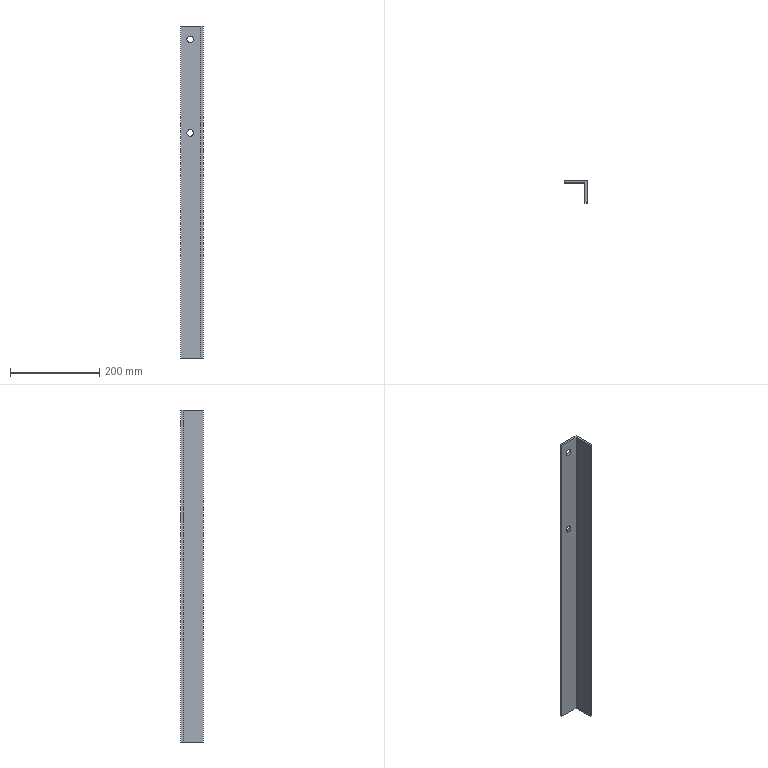Part | 1 solid | 12 faces | box 50 x 50 x 745 mm | volume 352108 mm3 | plane 8 | cylinder 4 | commonest cylinder face diameters 15 x4
STEP:
#1=CARTESIAN_POINT('',(21.,45.,497.5));
#2=VERTEX_POINT('',#1);
#3=CARTESIAN_POINT('',(21.,45.,512.5));
#4=VERTEX_POINT('',#3);
#5=CARTESIAN_POINT('',(21.,45.,505.));
#6=DIRECTION('',(0.,1.,0.));
#7=DIRECTION('',(0.,0.,1.));
#8=AXIS2_PLACEMENT_3D('',#5,#6,#7);
#9=CIRCLE('',#8,7.5);
#10=EDGE_CURVE('',#2,#4,#9,.T.);
#11=ORIENTED_EDGE('',*,*,#10,.F.);
#12=CARTESIAN_POINT('',(21.,50.,497.5));
#13=VERTEX_POINT('',#12);
#14=CARTESIAN_POINT('',(21.,0.,497.5));
#15=DIRECTION('',(0.,1.,0.));
#16=VECTOR('',#15,1000.);
#17=LINE('',#14,#16);
#18=EDGE_CURVE('',#2,#13,#17,.T.);
#19=ORIENTED_EDGE('',*,*,#18,.T.);
#20=CARTESIAN_POINT('',(21.,50.,512.5));
#21=VERTEX_POINT('',#20);
#22=CARTESIAN_POINT('',(21.,50.,505.));
#23=DIRECTION('',(0.,1.,0.));
#24=DIRECTION('',(0.,0.,1.));
#25=AXIS2_PLACEMENT_3D('',#22,#23,#24);
#26=CIRCLE('',#25,7.5);
#27=EDGE_CURVE('',#13,#21,#26,.T.);
#28=ORIENTED_EDGE('',*,*,#27,.T.);
#29=CARTESIAN_POINT('',(21.,0.,512.5));
#30=DIRECTION('',(0.,1.,0.));
#31=VECTOR('',#30,1000.);
#32=LINE('',#29,#31);
#33=EDGE_CURVE('',#4,#21,#32,.T.);
#34=ORIENTED_EDGE('',*,*,#33,.F.);
#35=EDGE_LOOP('',(#11,#19,#28,#34));
#36=FACE_OUTER_BOUND('',#35,.T.);
#37=CARTESIAN_POINT('',(21.,0.,505.));
#38=DIRECTION('',(0.,1.,0.));
#39=DIRECTION('',(0.,0.,1.));
#40=AXIS2_PLACEMENT_3D('',#37,#38,#39);
#41=CYLINDRICAL_SURFACE('',#40,7.5);
#42=ADVANCED_FACE('',(#36),#41,.F.);
#43=CARTESIAN_POINT('',(21.,45.,707.5));
#44=VERTEX_POINT('',#43);
#45=CARTESIAN_POINT('',(21.,45.,722.5));
#46=VERTEX_POINT('',#45);
#47=CARTESIAN_POINT('',(21.,45.,715.));
#48=DIRECTION('',(0.,1.,0.));
#49=DIRECTION('',(0.,0.,1.));
#50=AXIS2_PLACEMENT_3D('',#47,#48,#49);
#51=CIRCLE('',#50,7.5);
#52=EDGE_CURVE('',#44,#46,#51,.T.);
#53=ORIENTED_EDGE('',*,*,#52,.F.);
#54=CARTESIAN_POINT('',(21.,50.,707.5));
#55=VERTEX_POINT('',#54);
#56=CARTESIAN_POINT('',(21.,0.,707.5));
#57=DIRECTION('',(0.,1.,0.));
#58=VECTOR('',#57,1000.);
#59=LINE('',#56,#58);
#60=EDGE_CURVE('',#44,#55,#59,.T.);
#61=ORIENTED_EDGE('',*,*,#60,.T.);
#62=CARTESIAN_POINT('',(21.,50.,722.5));
#63=VERTEX_POINT('',#62);
#64=CARTESIAN_POINT('',(21.,50.,715.));
#65=DIRECTION('',(0.,1.,0.));
#66=DIRECTION('',(0.,0.,1.));
#67=AXIS2_PLACEMENT_3D('',#64,#65,#66);
#68=CIRCLE('',#67,7.5);
#69=EDGE_CURVE('',#55,#63,#68,.T.);
#70=ORIENTED_EDGE('',*,*,#69,.T.);
#71=CARTESIAN_POINT('',(21.,0.,722.5));
#72=DIRECTION('',(0.,1.,0.));
#73=VECTOR('',#72,1000.);
#74=LINE('',#71,#73);
#75=EDGE_CURVE('',#46,#63,#74,.T.);
#76=ORIENTED_EDGE('',*,*,#75,.F.);
#77=EDGE_LOOP('',(#53,#61,#70,#76));
#78=FACE_OUTER_BOUND('',#77,.T.);
#79=CARTESIAN_POINT('',(21.,0.,715.));
#80=DIRECTION('',(0.,1.,0.));
#81=DIRECTION('',(0.,0.,1.));
#82=AXIS2_PLACEMENT_3D('',#79,#80,#81);
#83=CYLINDRICAL_SURFACE('',#82,7.5);
#84=ADVANCED_FACE('',(#78),#83,.F.);
#85=CARTESIAN_POINT('',(0.,50.,0.));
#86=VERTEX_POINT('',#85);
#87=CARTESIAN_POINT('',(0.,45.,0.));
#88=VERTEX_POINT('',#87);
#89=CARTESIAN_POINT('',(0.,0.,0.));
#90=DIRECTION('',(0.,-1.,0.));
#91=VECTOR('',#90,1000.);
#92=LINE('',#89,#91);
#93=EDGE_CURVE('',#86,#88,#92,.T.);
#94=ORIENTED_EDGE('',*,*,#93,.T.);
#95=CARTESIAN_POINT('',(0.,45.,745.));
#96=VERTEX_POINT('',#95);
#97=CARTESIAN_POINT('',(0.,45.,0.));
#98=DIRECTION('',(0.,0.,1.));
#99=VECTOR('',#98,1000.);
#100=LINE('',#97,#99);
#101=EDGE_CURVE('',#88,#96,#100,.T.);
#102=ORIENTED_EDGE('',*,*,#101,.T.);
#103=CARTESIAN_POINT('',(0.,50.,745.));
#104=VERTEX_POINT('',#103);
#105=CARTESIAN_POINT('',(0.,0.,745.));
#106=DIRECTION('',(0.,-1.,0.));
#107=VECTOR('',#106,1000.);
#108=LINE('',#105,#107);
#109=EDGE_CURVE('',#104,#96,#108,.T.);
#110=ORIENTED_EDGE('',*,*,#109,.F.);
#111=CARTESIAN_POINT('',(0.,50.,760.));
#112=DIRECTION('',(0.,0.,-1.));
#113=VECTOR('',#112,1000.);
#114=LINE('',#111,#113);
#115=EDGE_CURVE('',#104,#86,#114,.T.);
#116=ORIENTED_EDGE('',*,*,#115,.T.);
#117=EDGE_LOOP('',(#94,#102,#110,#116));
#118=FACE_OUTER_BOUND('',#117,.T.);
#119=CARTESIAN_POINT('',(0.,0.,760.));
#120=DIRECTION('',(1.,0.,0.));
#121=DIRECTION('',(0.,1.,0.));
#122=AXIS2_PLACEMENT_3D('',#119,#120,#121);
#123=PLANE('',#122);
#124=ADVANCED_FACE('',(#118),#123,.F.);
#125=CARTESIAN_POINT('',(45.,0.,745.));
#126=VERTEX_POINT('',#125);
#127=CARTESIAN_POINT('',(50.,0.,745.));
#128=VERTEX_POINT('',#127);
#129=CARTESIAN_POINT('',(0.,0.,745.));
#130=DIRECTION('',(1.,0.,0.));
#131=VECTOR('',#130,1000.);
#132=LINE('',#129,#131);
#133=EDGE_CURVE('',#126,#128,#132,.T.);
#134=ORIENTED_EDGE('',*,*,#133,.F.);
#135=CARTESIAN_POINT('',(45.,0.,0.));
#136=VERTEX_POINT('',#135);
#137=CARTESIAN_POINT('',(45.,0.,0.));
#138=DIRECTION('',(0.,0.,1.));
#139=VECTOR('',#138,1000.);
#140=LINE('',#137,#139);
#141=EDGE_CURVE('',#136,#126,#140,.T.);
#142=ORIENTED_EDGE('',*,*,#141,.F.);
#143=CARTESIAN_POINT('',(50.,0.,0.));
#144=VERTEX_POINT('',#143);
#145=CARTESIAN_POINT('',(0.,0.,0.));
#146=DIRECTION('',(1.,0.,0.));
#147=VECTOR('',#146,1000.);
#148=LINE('',#145,#147);
#149=EDGE_CURVE('',#136,#144,#148,.T.);
#150=ORIENTED_EDGE('',*,*,#149,.T.);
#151=CARTESIAN_POINT('',(50.,0.,760.));
#152=DIRECTION('',(0.,0.,-1.));
#153=VECTOR('',#152,1000.);
#154=LINE('',#151,#153);
#155=EDGE_CURVE('',#128,#144,#154,.T.);
#156=ORIENTED_EDGE('',*,*,#155,.F.);
#157=EDGE_LOOP('',(#134,#142,#150,#156));
#158=FACE_OUTER_BOUND('',#157,.T.);
#159=CARTESIAN_POINT('',(0.,0.,760.));
#160=DIRECTION('',(0.,1.,0.));
#161=DIRECTION('',(0.,0.,1.));
#162=AXIS2_PLACEMENT_3D('',#159,#160,#161);
#163=PLANE('',#162);
#164=ADVANCED_FACE('',(#158),#163,.F.);
#165=CARTESIAN_POINT('',(50.,50.,0.));
#166=VERTEX_POINT('',#165);
#167=CARTESIAN_POINT('',(50.,0.,0.));
#168=DIRECTION('',(0.,1.,0.));
#169=VECTOR('',#168,1000.);
#170=LINE('',#167,#169);
#171=EDGE_CURVE('',#144,#166,#170,.T.);
#172=ORIENTED_EDGE('',*,*,#171,.T.);
#173=CARTESIAN_POINT('',(50.,50.,745.));
#174=VERTEX_POINT('',#173);
#175=CARTESIAN_POINT('',(50.,50.,760.));
#176=DIRECTION('',(0.,0.,-1.));
#177=VECTOR('',#176,1000.);
#178=LINE('',#175,#177);
#179=EDGE_CURVE('',#174,#166,#178,.T.);
#180=ORIENTED_EDGE('',*,*,#179,.F.);
#181=CARTESIAN_POINT('',(50.,0.,745.));
#182=DIRECTION('',(0.,1.,0.));
#183=VECTOR('',#182,1000.);
#184=LINE('',#181,#183);
#185=EDGE_CURVE('',#128,#174,#184,.T.);
#186=ORIENTED_EDGE('',*,*,#185,.F.);
#187=ORIENTED_EDGE('',*,*,#155,.T.);
#188=EDGE_LOOP('',(#172,#180,#186,#187));
#189=FACE_OUTER_BOUND('',#188,.T.);
#190=CARTESIAN_POINT('',(50.,0.,760.));
#191=DIRECTION('',(-1.,0.,0.));
#192=DIRECTION('',(0.,-1.,0.));
#193=AXIS2_PLACEMENT_3D('',#190,#191,#192);
#194=PLANE('',#193);
#195=ADVANCED_FACE('',(#189),#194,.F.);
#196=CARTESIAN_POINT('',(21.,50.,505.));
#197=DIRECTION('',(0.,1.,0.));
#198=DIRECTION('',(0.,0.,1.));
#199=AXIS2_PLACEMENT_3D('',#196,#197,#198);
#200=CIRCLE('',#199,7.5);
#201=EDGE_CURVE('',#21,#13,#200,.T.);
#202=ORIENTED_EDGE('',*,*,#201,.F.);
#203=ORIENTED_EDGE('',*,*,#27,.F.);
#204=EDGE_LOOP('',(#202,#203));
#205=FACE_BOUND('',#204,.T.);
#206=CARTESIAN_POINT('',(21.,50.,715.));
#207=DIRECTION('',(0.,1.,0.));
#208=DIRECTION('',(0.,0.,1.));
#209=AXIS2_PLACEMENT_3D('',#206,#207,#208);
#210=CIRCLE('',#209,7.5);
#211=EDGE_CURVE('',#63,#55,#210,.T.);
#212=ORIENTED_EDGE('',*,*,#211,.F.);
#213=ORIENTED_EDGE('',*,*,#69,.F.);
#214=EDGE_LOOP('',(#212,#213));
#215=FACE_BOUND('',#214,.T.);
#216=CARTESIAN_POINT('',(0.,50.,0.));
#217=DIRECTION('',(-1.,0.,0.));
#218=VECTOR('',#217,1000.);
#219=LINE('',#216,#218);
#220=EDGE_CURVE('',#166,#86,#219,.T.);
#221=ORIENTED_EDGE('',*,*,#220,.T.);
#222=ORIENTED_EDGE('',*,*,#115,.F.);
#223=CARTESIAN_POINT('',(0.,50.,745.));
#224=DIRECTION('',(-1.,0.,0.));
#225=VECTOR('',#224,1000.);
#226=LINE('',#223,#225);
#227=EDGE_CURVE('',#174,#104,#226,.T.);
#228=ORIENTED_EDGE('',*,*,#227,.F.);
#229=ORIENTED_EDGE('',*,*,#179,.T.);
#230=EDGE_LOOP('',(#221,#222,#228,#229));
#231=FACE_OUTER_BOUND('',#230,.T.);
#232=CARTESIAN_POINT('',(0.,50.,760.));
#233=DIRECTION('',(0.,-1.,0.));
#234=DIRECTION('',(0.,0.,-1.));
#235=AXIS2_PLACEMENT_3D('',#232,#233,#234);
#236=PLANE('',#235);
#237=ADVANCED_FACE('',(#205,#215,#231),#236,.F.);
#238=ORIENTED_EDGE('',*,*,#109,.T.);
#239=CARTESIAN_POINT('',(45.,45.,745.));
#240=VERTEX_POINT('',#239);
#241=CARTESIAN_POINT('',(0.,45.,745.));
#242=DIRECTION('',(-1.,0.,0.));
#243=VECTOR('',#242,1000.);
#244=LINE('',#241,#243);
#245=EDGE_CURVE('',#240,#96,#244,.T.);
#246=ORIENTED_EDGE('',*,*,#245,.F.);
#247=CARTESIAN_POINT('',(45.,0.,745.));
#248=DIRECTION('',(0.,1.,0.));
#249=VECTOR('',#248,1000.);
#250=LINE('',#247,#249);
#251=EDGE_CURVE('',#126,#240,#250,.T.);
#252=ORIENTED_EDGE('',*,*,#251,.F.);
#253=ORIENTED_EDGE('',*,*,#133,.T.);
#254=ORIENTED_EDGE('',*,*,#185,.T.);
#255=ORIENTED_EDGE('',*,*,#227,.T.);
#256=EDGE_LOOP('',(#238,#246,#252,#253,#254,#255));
#257=FACE_OUTER_BOUND('',#256,.T.);
#258=CARTESIAN_POINT('',(0.,0.,745.));
#259=DIRECTION('',(0.,0.,-1.));
#260=DIRECTION('',(-1.,0.,0.));
#261=AXIS2_PLACEMENT_3D('',#258,#259,#260);
#262=PLANE('',#261);
#263=ADVANCED_FACE('',(#257),#262,.F.);
#264=CARTESIAN_POINT('',(45.,45.,0.));
#265=VERTEX_POINT('',#264);
#266=CARTESIAN_POINT('',(0.,45.,0.));
#267=DIRECTION('',(-1.,0.,0.));
#268=VECTOR('',#267,1000.);
#269=LINE('',#266,#268);
#270=EDGE_CURVE('',#265,#88,#269,.T.);
#271=ORIENTED_EDGE('',*,*,#270,.T.);
#272=ORIENTED_EDGE('',*,*,#93,.F.);
#273=ORIENTED_EDGE('',*,*,#220,.F.);
#274=ORIENTED_EDGE('',*,*,#171,.F.);
#275=ORIENTED_EDGE('',*,*,#149,.F.);
#276=CARTESIAN_POINT('',(45.,0.,0.));
#277=DIRECTION('',(0.,1.,0.));
#278=VECTOR('',#277,1000.);
#279=LINE('',#276,#278);
#280=EDGE_CURVE('',#136,#265,#279,.T.);
#281=ORIENTED_EDGE('',*,*,#280,.T.);
#282=EDGE_LOOP('',(#271,#272,#273,#274,#275,#281));
#283=FACE_OUTER_BOUND('',#282,.T.);
#284=CARTESIAN_POINT('',(0.,0.,0.));
#285=DIRECTION('',(0.,0.,-1.));
#286=DIRECTION('',(-1.,0.,0.));
#287=AXIS2_PLACEMENT_3D('',#284,#285,#286);
#288=PLANE('',#287);
#289=ADVANCED_FACE('',(#283),#288,.T.);
#290=CARTESIAN_POINT('',(21.,45.,505.));
#291=DIRECTION('',(0.,1.,0.));
#292=DIRECTION('',(0.,0.,1.));
#293=AXIS2_PLACEMENT_3D('',#290,#291,#292);
#294=CIRCLE('',#293,7.5);
#295=EDGE_CURVE('',#4,#2,#294,.T.);
#296=ORIENTED_EDGE('',*,*,#295,.T.);
#297=ORIENTED_EDGE('',*,*,#10,.T.);
#298=EDGE_LOOP('',(#296,#297));
#299=FACE_BOUND('',#298,.T.);
#300=CARTESIAN_POINT('',(21.,45.,715.));
#301=DIRECTION('',(0.,1.,0.));
#302=DIRECTION('',(0.,0.,1.));
#303=AXIS2_PLACEMENT_3D('',#300,#301,#302);
#304=CIRCLE('',#303,7.5);
#305=EDGE_CURVE('',#46,#44,#304,.T.);
#306=ORIENTED_EDGE('',*,*,#305,.T.);
#307=ORIENTED_EDGE('',*,*,#52,.T.);
#308=EDGE_LOOP('',(#306,#307));
#309=FACE_BOUND('',#308,.T.);
#310=ORIENTED_EDGE('',*,*,#245,.T.);
#311=ORIENTED_EDGE('',*,*,#101,.F.);
#312=ORIENTED_EDGE('',*,*,#270,.F.);
#313=CARTESIAN_POINT('',(45.,45.,0.));
#314=DIRECTION('',(0.,0.,1.));
#315=VECTOR('',#314,1000.);
#316=LINE('',#313,#315);
#317=EDGE_CURVE('',#265,#240,#316,.T.);
#318=ORIENTED_EDGE('',*,*,#317,.T.);
#319=EDGE_LOOP('',(#310,#311,#312,#318));
#320=FACE_OUTER_BOUND('',#319,.T.);
#321=CARTESIAN_POINT('',(0.,45.,0.));
#322=DIRECTION('',(0.,1.,0.));
#323=DIRECTION('',(0.,0.,1.));
#324=AXIS2_PLACEMENT_3D('',#321,#322,#323);
#325=PLANE('',#324);
#326=ADVANCED_FACE('',(#299,#309,#320),#325,.F.);
#327=ORIENTED_EDGE('',*,*,#251,.T.);
#328=ORIENTED_EDGE('',*,*,#317,.F.);
#329=ORIENTED_EDGE('',*,*,#280,.F.);
#330=ORIENTED_EDGE('',*,*,#141,.T.);
#331=EDGE_LOOP('',(#327,#328,#329,#330));
#332=FACE_OUTER_BOUND('',#331,.T.);
#333=CARTESIAN_POINT('',(45.,0.,0.));
#334=DIRECTION('',(1.,0.,0.));
#335=DIRECTION('',(0.,1.,0.));
#336=AXIS2_PLACEMENT_3D('',#333,#334,#335);
#337=PLANE('',#336);
#338=ADVANCED_FACE('',(#332),#337,.F.);
#339=ORIENTED_EDGE('',*,*,#60,.F.);
#340=ORIENTED_EDGE('',*,*,#305,.F.);
#341=ORIENTED_EDGE('',*,*,#75,.T.);
#342=ORIENTED_EDGE('',*,*,#211,.T.);
#343=EDGE_LOOP('',(#339,#340,#341,#342));
#344=FACE_OUTER_BOUND('',#343,.T.);
#345=CARTESIAN_POINT('',(21.,0.,715.));
#346=DIRECTION('',(0.,1.,0.));
#347=DIRECTION('',(0.,0.,1.));
#348=AXIS2_PLACEMENT_3D('',#345,#346,#347);
#349=CYLINDRICAL_SURFACE('',#348,7.5);
#350=ADVANCED_FACE('',(#344),#349,.F.);
#351=ORIENTED_EDGE('',*,*,#18,.F.);
#352=ORIENTED_EDGE('',*,*,#295,.F.);
#353=ORIENTED_EDGE('',*,*,#33,.T.);
#354=ORIENTED_EDGE('',*,*,#201,.T.);
#355=EDGE_LOOP('',(#351,#352,#353,#354));
#356=FACE_OUTER_BOUND('',#355,.T.);
#357=CARTESIAN_POINT('',(21.,0.,505.));
#358=DIRECTION('',(0.,1.,0.));
#359=DIRECTION('',(0.,0.,1.));
#360=AXIS2_PLACEMENT_3D('',#357,#358,#359);
#361=CYLINDRICAL_SURFACE('',#360,7.5);
#362=ADVANCED_FACE('',(#356),#361,.F.);
#363=CLOSED_SHELL('',(#42,#84,#124,#164,#195,#237,#263,#289,#326,#338,#350,#362));
#364=MANIFOLD_SOLID_BREP('',#363);
#365=CARTESIAN_POINT('',(0.,0.,0.));
#366=DIRECTION('',(0.,0.,1.));
#367=DIRECTION('',(1.,0.,0.));
#368=AXIS2_PLACEMENT_3D('',#365,#366,#367);
#369=(LENGTH_UNIT()NAMED_UNIT(*)SI_UNIT(.MILLI.,.METRE.));
#370=UNCERTAINTY_MEASURE_WITH_UNIT(LENGTH_MEASURE(0.00001),#369,'','');
#371=(NAMED_UNIT(*)PLANE_ANGLE_UNIT()SI_UNIT($,.RADIAN.));
#372=(NAMED_UNIT(*)SI_UNIT($,.STERADIAN.)SOLID_ANGLE_UNIT());
#373=(GEOMETRIC_REPRESENTATION_CONTEXT(3)GLOBAL_UNCERTAINTY_ASSIGNED_CONTEXT((#370))GLOBAL_UNIT_ASSIGNED_CONTEXT((#369,#371,#372))REPRESENTATION_CONTEXT('',''));
#374=ADVANCED_BREP_SHAPE_REPRESENTATION('',(#364,#368),#373);